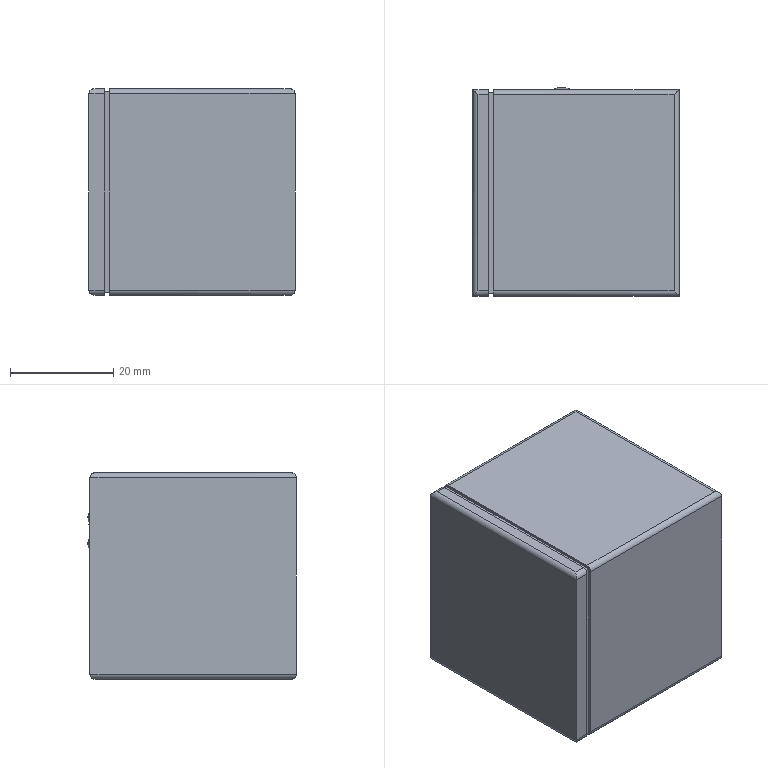Part | SolidWorks | features BaseBody 1 | 1 solid | 32 faces | box 40 x 40.45 x 40 mm | volume 63851 mm3 | plane 16 | cylinder 12 | spline 4 | commonest cylinder face diameters 2 x12
STEP:
#1=CARTESIAN_POINT('',(19.153,20.,6.3));
#2=VERTEX_POINT('',#1);
#3=CARTESIAN_POINT('',(15.347,20.,6.3));
#4=VERTEX_POINT('',#3);
#5=CARTESIAN_POINT('',(19.153,20.,6.3));
#6=CARTESIAN_POINT('',(19.153,20.,6.426));
#7=CARTESIAN_POINT('',(19.141,20.,6.549));
#8=CARTESIAN_POINT('',(19.093,20.,6.792));
#9=CARTESIAN_POINT('',(19.056,20.,6.913));
#10=CARTESIAN_POINT('',(18.961,20.,7.144));
#11=CARTESIAN_POINT('',(18.902,20.,7.253));
#12=CARTESIAN_POINT('',(18.764,20.,7.46));
#13=CARTESIAN_POINT('',(18.684,20.,7.558));
#14=CARTESIAN_POINT('',(18.421,20.,7.821));
#15=CARTESIAN_POINT('',(18.209,20.,7.963));
#16=CARTESIAN_POINT('',(17.751,20.,8.153));
#17=CARTESIAN_POINT('',(17.501,20.,8.203));
#18=CARTESIAN_POINT('',(17.124,20.,8.203));
#19=CARTESIAN_POINT('',(17.001,20.,8.191));
#20=CARTESIAN_POINT('',(16.758,20.,8.143));
#21=CARTESIAN_POINT('',(16.637,20.,8.106));
#22=CARTESIAN_POINT('',(16.406,20.,8.011));
#23=CARTESIAN_POINT('',(16.297,20.,7.952));
#24=CARTESIAN_POINT('',(16.09,20.,7.814));
#25=CARTESIAN_POINT('',(15.992,20.,7.734));
#26=CARTESIAN_POINT('',(15.729,20.,7.471));
#27=CARTESIAN_POINT('',(15.587,20.,7.259));
#28=CARTESIAN_POINT('',(15.397,20.,6.801));
#29=CARTESIAN_POINT('',(15.347,20.,6.551));
#30=CARTESIAN_POINT('',(15.347,20.,6.3));
#31=B_SPLINE_CURVE_WITH_KNOTS('',3,(#5,#6,#7,#8,#9,#10,#11,#12,#13,#14,#15,#16,#17,#18,#19,#20,#21,#22,#23,#24,#25,#26,#27,#28,#29,#30),.UNSPECIFIED.,.F.,.F.,(4,2,2,2,2,2,2,2,2,2,2,2,4),(0.,0.0003717,0.0007433,0.001115,0.001487,0.00223,0.002973,0.003345,0.003717,0.004088,0.00446,0.005203,0.005946),.UNSPECIFIED.);
#32=EDGE_CURVE('',#2,#4,#31,.T.);
#33=ORIENTED_EDGE('',*,*,#32,.F.);
#34=CARTESIAN_POINT('',(17.25,16.2,6.3));
#35=DIRECTION('',(0.,0.,1.));
#36=DIRECTION('',(1.,0.,0.));
#37=AXIS2_PLACEMENT_3D('',#34,#35,#36);
#38=CIRCLE('',#37,4.25);
#39=EDGE_CURVE('',#2,#4,#38,.T.);
#40=ORIENTED_EDGE('',*,*,#39,.T.);
#41=EDGE_LOOP('',(#33,#40));
#42=FACE_OUTER_BOUND('',#41,.T.);
#43=CARTESIAN_POINT('',(19.174,19.989,6.3));
#44=CARTESIAN_POINT('',(19.174,19.989,6.895));
#45=CARTESIAN_POINT('',(19.174,19.852,7.475));
#46=CARTESIAN_POINT('',(19.174,19.583,8.006));
#47=CARTESIAN_POINT('',(17.941,20.616,6.3));
#48=CARTESIAN_POINT('',(17.941,20.616,6.994));
#49=CARTESIAN_POINT('',(17.941,20.455,7.669));
#50=CARTESIAN_POINT('',(17.941,20.142,8.288));
#51=CARTESIAN_POINT('',(16.559,20.616,6.3));
#52=CARTESIAN_POINT('',(16.559,20.616,6.994));
#53=CARTESIAN_POINT('',(16.559,20.455,7.669));
#54=CARTESIAN_POINT('',(16.559,20.142,8.288));
#55=CARTESIAN_POINT('',(15.326,19.989,6.3));
#56=CARTESIAN_POINT('',(15.326,19.989,6.895));
#57=CARTESIAN_POINT('',(15.326,19.852,7.475));
#58=CARTESIAN_POINT('',(15.326,19.583,8.006));
#59=(BOUNDED_SURFACE()B_SPLINE_SURFACE(3,3,((#43,#44,#45,#46),(#47,#48,#49,#50),(#51,#52,#53,#54),(#55,#56,#57,#58)),.UNSPECIFIED.,.F.,.F.,.F.)B_SPLINE_SURFACE_WITH_KNOTS((4,4),(4,4),(0.,1.),(0.,1.),.UNSPECIFIED.)GEOMETRIC_REPRESENTATION_ITEM()RATIONAL_B_SPLINE_SURFACE(((1.,0.9819,0.9819,1.),(0.9277,0.9109,0.9109,0.9277),(0.9277,0.9109,0.9109,0.9277),(1.,0.9819,0.9819,1.)))REPRESENTATION_ITEM('')SURFACE());
#60=ADVANCED_FACE('',(#42),#59,.T.);
#61=CARTESIAN_POINT('',(19.153,20.,11.3));
#62=VERTEX_POINT('',#61);
#63=CARTESIAN_POINT('',(15.347,20.,11.3));
#64=VERTEX_POINT('',#63);
#65=CARTESIAN_POINT('',(19.153,20.,11.3));
#66=CARTESIAN_POINT('',(19.153,20.,11.426));
#67=CARTESIAN_POINT('',(19.141,20.,11.549));
#68=CARTESIAN_POINT('',(19.093,20.,11.792));
#69=CARTESIAN_POINT('',(19.056,20.,11.913));
#70=CARTESIAN_POINT('',(18.961,20.,12.144));
#71=CARTESIAN_POINT('',(18.902,20.,12.253));
#72=CARTESIAN_POINT('',(18.764,20.,12.46));
#73=CARTESIAN_POINT('',(18.684,20.,12.558));
#74=CARTESIAN_POINT('',(18.421,20.,12.821));
#75=CARTESIAN_POINT('',(18.209,20.,12.963));
#76=CARTESIAN_POINT('',(17.751,20.,13.153));
#77=CARTESIAN_POINT('',(17.501,20.,13.203));
#78=CARTESIAN_POINT('',(17.124,20.,13.203));
#79=CARTESIAN_POINT('',(17.001,20.,13.191));
#80=CARTESIAN_POINT('',(16.758,20.,13.143));
#81=CARTESIAN_POINT('',(16.637,20.,13.106));
#82=CARTESIAN_POINT('',(16.406,20.,13.011));
#83=CARTESIAN_POINT('',(16.297,20.,12.952));
#84=CARTESIAN_POINT('',(16.09,20.,12.814));
#85=CARTESIAN_POINT('',(15.992,20.,12.734));
#86=CARTESIAN_POINT('',(15.729,20.,12.471));
#87=CARTESIAN_POINT('',(15.587,20.,12.259));
#88=CARTESIAN_POINT('',(15.397,20.,11.801));
#89=CARTESIAN_POINT('',(15.347,20.,11.551));
#90=CARTESIAN_POINT('',(15.347,20.,11.3));
#91=B_SPLINE_CURVE_WITH_KNOTS('',3,(#65,#66,#67,#68,#69,#70,#71,#72,#73,#74,#75,#76,#77,#78,#79,#80,#81,#82,#83,#84,#85,#86,#87,#88,#89,#90),.UNSPECIFIED.,.F.,.F.,(4,2,2,2,2,2,2,2,2,2,2,2,4),(0.,0.0003717,0.0007433,0.001115,0.001487,0.00223,0.002973,0.003345,0.003717,0.004088,0.00446,0.005203,0.005946),.UNSPECIFIED.);
#92=EDGE_CURVE('',#62,#64,#91,.T.);
#93=ORIENTED_EDGE('',*,*,#92,.F.);
#94=CARTESIAN_POINT('',(17.25,16.2,11.3));
#95=DIRECTION('',(0.,0.,1.));
#96=DIRECTION('',(1.,0.,0.));
#97=AXIS2_PLACEMENT_3D('',#94,#95,#96);
#98=CIRCLE('',#97,4.25);
#99=EDGE_CURVE('',#62,#64,#98,.T.);
#100=ORIENTED_EDGE('',*,*,#99,.T.);
#101=EDGE_LOOP('',(#93,#100));
#102=FACE_OUTER_BOUND('',#101,.T.);
#103=CARTESIAN_POINT('',(19.174,19.989,11.3));
#104=CARTESIAN_POINT('',(19.174,19.989,11.895));
#105=CARTESIAN_POINT('',(19.174,19.852,12.475));
#106=CARTESIAN_POINT('',(19.174,19.583,13.006));
#107=CARTESIAN_POINT('',(17.941,20.616,11.3));
#108=CARTESIAN_POINT('',(17.941,20.616,11.994));
#109=CARTESIAN_POINT('',(17.941,20.455,12.669));
#110=CARTESIAN_POINT('',(17.941,20.142,13.288));
#111=CARTESIAN_POINT('',(16.559,20.616,11.3));
#112=CARTESIAN_POINT('',(16.559,20.616,11.994));
#113=CARTESIAN_POINT('',(16.559,20.455,12.669));
#114=CARTESIAN_POINT('',(16.559,20.142,13.288));
#115=CARTESIAN_POINT('',(15.326,19.989,11.3));
#116=CARTESIAN_POINT('',(15.326,19.989,11.895));
#117=CARTESIAN_POINT('',(15.326,19.852,12.475));
#118=CARTESIAN_POINT('',(15.326,19.583,13.006));
#119=(BOUNDED_SURFACE()B_SPLINE_SURFACE(3,3,((#103,#104,#105,#106),(#107,#108,#109,#110),(#111,#112,#113,#114),(#115,#116,#117,#118)),.UNSPECIFIED.,.F.,.F.,.F.)B_SPLINE_SURFACE_WITH_KNOTS((4,4),(4,4),(0.,1.),(0.,1.),.UNSPECIFIED.)GEOMETRIC_REPRESENTATION_ITEM()RATIONAL_B_SPLINE_SURFACE(((1.,0.9819,0.9819,1.),(0.9277,0.9109,0.9109,0.9277),(0.9277,0.9109,0.9109,0.9277),(1.,0.9819,0.9819,1.)))REPRESENTATION_ITEM('')SURFACE());
#120=ADVANCED_FACE('',(#102),#119,.T.);
#121=CARTESIAN_POINT('',(40.,20.,19.));
#122=VERTEX_POINT('',#121);
#123=CARTESIAN_POINT('',(40.,-20.,19.));
#124=VERTEX_POINT('',#123);
#125=CARTESIAN_POINT('',(40.,20.,19.));
#126=DIRECTION('',(0.,-1.,0.));
#127=VECTOR('',#126,1000.);
#128=LINE('',#125,#127);
#129=EDGE_CURVE('',#122,#124,#128,.T.);
#130=ORIENTED_EDGE('',*,*,#129,.T.);
#131=CARTESIAN_POINT('',(40.,-20.,-19.));
#132=VERTEX_POINT('',#131);
#133=CARTESIAN_POINT('',(40.,-20.,19.));
#134=DIRECTION('',(0.,0.,-1.));
#135=VECTOR('',#134,1000.);
#136=LINE('',#133,#135);
#137=EDGE_CURVE('',#124,#132,#136,.T.);
#138=ORIENTED_EDGE('',*,*,#137,.T.);
#139=CARTESIAN_POINT('',(40.,20.,-19.));
#140=VERTEX_POINT('',#139);
#141=CARTESIAN_POINT('',(40.,20.,-19.));
#142=DIRECTION('',(0.,1.,0.));
#143=VECTOR('',#142,1000.);
#144=LINE('',#141,#143);
#145=EDGE_CURVE('',#132,#140,#144,.T.);
#146=ORIENTED_EDGE('',*,*,#145,.T.);
#147=CARTESIAN_POINT('',(40.,20.,19.));
#148=DIRECTION('',(0.,0.,1.));
#149=VECTOR('',#148,1000.);
#150=LINE('',#147,#149);
#151=EDGE_CURVE('',#140,#122,#150,.T.);
#152=ORIENTED_EDGE('',*,*,#151,.T.);
#153=EDGE_LOOP('',(#130,#138,#146,#152));
#154=FACE_OUTER_BOUND('',#153,.T.);
#155=CARTESIAN_POINT('',(40.,20.,19.));
#156=DIRECTION('',(1.,0.,0.));
#157=DIRECTION('',(0.,0.,-1.));
#158=AXIS2_PLACEMENT_3D('',#155,#156,#157);
#159=PLANE('',#158);
#160=ADVANCED_FACE('',(#154),#159,.T.);
#161=ORIENTED_EDGE('',*,*,#137,.F.);
#162=CARTESIAN_POINT('',(4.,-20.,19.));
#163=VERTEX_POINT('',#162);
#164=CARTESIAN_POINT('',(0.,-20.,19.));
#165=DIRECTION('',(1.,0.,0.));
#166=VECTOR('',#165,1000.);
#167=LINE('',#164,#166);
#168=EDGE_CURVE('',#163,#124,#167,.T.);
#169=ORIENTED_EDGE('',*,*,#168,.F.);
#170=CARTESIAN_POINT('',(4.,-20.,-19.));
#171=VERTEX_POINT('',#170);
#172=CARTESIAN_POINT('',(4.,-20.,0.));
#173=DIRECTION('',(0.,0.,1.));
#174=VECTOR('',#173,1000.);
#175=LINE('',#172,#174);
#176=EDGE_CURVE('',#171,#163,#175,.T.);
#177=ORIENTED_EDGE('',*,*,#176,.F.);
#178=CARTESIAN_POINT('',(0.,-20.,-19.));
#179=DIRECTION('',(-1.,0.,0.));
#180=VECTOR('',#179,1000.);
#181=LINE('',#178,#180);
#182=EDGE_CURVE('',#132,#171,#181,.T.);
#183=ORIENTED_EDGE('',*,*,#182,.F.);
#184=EDGE_LOOP('',(#161,#169,#177,#183));
#185=FACE_OUTER_BOUND('',#184,.T.);
#186=CARTESIAN_POINT('',(0.,-20.,0.));
#187=DIRECTION('',(0.,1.,0.));
#188=DIRECTION('',(0.,0.,1.));
#189=AXIS2_PLACEMENT_3D('',#186,#187,#188);
#190=PLANE('',#189);
#191=ADVANCED_FACE('',(#185),#190,.F.);
#192=ORIENTED_EDGE('',*,*,#129,.F.);
#193=CARTESIAN_POINT('',(39.,19.,20.));
#194=VERTEX_POINT('',#193);
#195=CARTESIAN_POINT('',(40.,20.,19.));
#196=CARTESIAN_POINT('',(40.,20.,19.586));
#197=CARTESIAN_POINT('',(39.586,19.586,20.));
#198=CARTESIAN_POINT('',(39.,19.,20.));
#199=(BOUNDED_CURVE()B_SPLINE_CURVE(3,(#195,#196,#197,#198),.UNSPECIFIED.,.F.,.F.)B_SPLINE_CURVE_WITH_KNOTS((4,4),(0.,1.571),.UNSPECIFIED.)CURVE()GEOMETRIC_REPRESENTATION_ITEM()RATIONAL_B_SPLINE_CURVE((1.,0.8047,0.8047,1.))REPRESENTATION_ITEM(''));
#200=EDGE_CURVE('',#122,#194,#199,.T.);
#201=ORIENTED_EDGE('',*,*,#200,.T.);
#202=CARTESIAN_POINT('',(39.,-19.,20.));
#203=VERTEX_POINT('',#202);
#204=CARTESIAN_POINT('',(39.,20.,20.));
#205=DIRECTION('',(0.,-1.,0.));
#206=VECTOR('',#205,1000.);
#207=LINE('',#204,#206);
#208=EDGE_CURVE('',#194,#203,#207,.T.);
#209=ORIENTED_EDGE('',*,*,#208,.T.);
#210=CARTESIAN_POINT('',(39.,-19.,20.));
#211=CARTESIAN_POINT('',(39.586,-19.586,20.));
#212=CARTESIAN_POINT('',(40.,-20.,19.586));
#213=CARTESIAN_POINT('',(40.,-20.,19.));
#214=(BOUNDED_CURVE()B_SPLINE_CURVE(3,(#210,#211,#212,#213),.UNSPECIFIED.,.F.,.F.)B_SPLINE_CURVE_WITH_KNOTS((4,4),(1.571,3.142),.UNSPECIFIED.)CURVE()GEOMETRIC_REPRESENTATION_ITEM()RATIONAL_B_SPLINE_CURVE((1.,0.8047,0.8047,1.))REPRESENTATION_ITEM(''));
#215=EDGE_CURVE('',#203,#124,#214,.T.);
#216=ORIENTED_EDGE('',*,*,#215,.T.);
#217=EDGE_LOOP('',(#192,#201,#209,#216));
#218=FACE_OUTER_BOUND('',#217,.T.);
#219=CARTESIAN_POINT('',(39.,20.,19.));
#220=DIRECTION('',(0.,1.,0.));
#221=DIRECTION('',(0.,0.,1.));
#222=AXIS2_PLACEMENT_3D('',#219,#220,#221);
#223=CYLINDRICAL_SURFACE('',#222,1.);
#224=ADVANCED_FACE('',(#218),#223,.T.);
#225=CARTESIAN_POINT('',(15.347,20.,6.3));
#226=CARTESIAN_POINT('',(15.347,20.,6.174));
#227=CARTESIAN_POINT('',(15.359,20.,6.051));
#228=CARTESIAN_POINT('',(15.407,20.,5.807));
#229=CARTESIAN_POINT('',(15.444,20.,5.687));
#230=CARTESIAN_POINT('',(15.539,20.,5.456));
#231=CARTESIAN_POINT('',(15.598,20.,5.347));
#232=CARTESIAN_POINT('',(15.736,20.,5.14));
#233=CARTESIAN_POINT('',(15.816,20.,5.042));
#234=CARTESIAN_POINT('',(16.08,20.,4.779));
#235=CARTESIAN_POINT('',(16.292,20.,4.637));
#236=CARTESIAN_POINT('',(16.75,20.,4.447));
#237=CARTESIAN_POINT('',(17.,20.,4.397));
#238=CARTESIAN_POINT('',(17.373,20.,4.397));
#239=CARTESIAN_POINT('',(17.499,20.,4.409));
#240=CARTESIAN_POINT('',(17.743,20.,4.457));
#241=CARTESIAN_POINT('',(17.862,20.,4.493));
#242=CARTESIAN_POINT('',(18.092,20.,4.589));
#243=CARTESIAN_POINT('',(18.204,20.,4.648));
#244=CARTESIAN_POINT('',(18.41,20.,4.786));
#245=CARTESIAN_POINT('',(18.506,20.,4.864));
#246=CARTESIAN_POINT('',(18.684,20.,5.042));
#247=CARTESIAN_POINT('',(18.763,20.,5.138));
#248=CARTESIAN_POINT('',(18.901,20.,5.344));
#249=CARTESIAN_POINT('',(18.96,20.,5.455));
#250=CARTESIAN_POINT('',(19.056,20.,5.686));
#251=CARTESIAN_POINT('',(19.092,20.,5.805));
#252=CARTESIAN_POINT('',(19.141,20.,6.048));
#253=CARTESIAN_POINT('',(19.153,20.,6.174));
#254=CARTESIAN_POINT('',(19.153,20.,6.3));
#255=B_SPLINE_CURVE_WITH_KNOTS('',3,(#225,#226,#227,#228,#229,#230,#231,#232,#233,#234,#235,#236,#237,#238,#239,#240,#241,#242,#243,#244,#245,#246,#247,#248,#249,#250,#251,#252,#253,#254),.UNSPECIFIED.,.F.,.F.,(4,2,2,2,2,2,2,2,2,2,2,2,2,2,4),(-0.005949,-0.005577,-0.005206,-0.004834,-0.004462,-0.003718,-0.002975,-0.002603,-0.002231,-0.001859,-0.001487,-0.001115,-0.0007437,-0.0003718,0.),.UNSPECIFIED.);
#256=EDGE_CURVE('',#4,#2,#255,.T.);
#257=ORIENTED_EDGE('',*,*,#256,.T.);
#258=ORIENTED_EDGE('',*,*,#32,.T.);
#259=EDGE_LOOP('',(#257,#258));
#260=FACE_BOUND('',#259,.T.);
#261=CARTESIAN_POINT('',(15.347,20.,11.3));
#262=CARTESIAN_POINT('',(15.347,20.,11.174));
#263=CARTESIAN_POINT('',(15.359,20.,11.051));
#264=CARTESIAN_POINT('',(15.407,20.,10.807));
#265=CARTESIAN_POINT('',(15.444,20.,10.687));
#266=CARTESIAN_POINT('',(15.539,20.,10.456));
#267=CARTESIAN_POINT('',(15.598,20.,10.347));
#268=CARTESIAN_POINT('',(15.736,20.,10.14));
#269=CARTESIAN_POINT('',(15.816,20.,10.042));
#270=CARTESIAN_POINT('',(16.08,20.,9.779));
#271=CARTESIAN_POINT('',(16.292,20.,9.637));
#272=CARTESIAN_POINT('',(16.75,20.,9.447));
#273=CARTESIAN_POINT('',(17.,20.,9.397));
#274=CARTESIAN_POINT('',(17.373,20.,9.397));
#275=CARTESIAN_POINT('',(17.499,20.,9.409));
#276=CARTESIAN_POINT('',(17.743,20.,9.457));
#277=CARTESIAN_POINT('',(17.862,20.,9.493));
#278=CARTESIAN_POINT('',(18.092,20.,9.589));
#279=CARTESIAN_POINT('',(18.204,20.,9.648));
#280=CARTESIAN_POINT('',(18.41,20.,9.786));
#281=CARTESIAN_POINT('',(18.506,20.,9.864));
#282=CARTESIAN_POINT('',(18.684,20.,10.042));
#283=CARTESIAN_POINT('',(18.763,20.,10.138));
#284=CARTESIAN_POINT('',(18.901,20.,10.344));
#285=CARTESIAN_POINT('',(18.96,20.,10.455));
#286=CARTESIAN_POINT('',(19.056,20.,10.686));
#287=CARTESIAN_POINT('',(19.092,20.,10.805));
#288=CARTESIAN_POINT('',(19.141,20.,11.048));
#289=CARTESIAN_POINT('',(19.153,20.,11.174));
#290=CARTESIAN_POINT('',(19.153,20.,11.3));
#291=B_SPLINE_CURVE_WITH_KNOTS('',3,(#261,#262,#263,#264,#265,#266,#267,#268,#269,#270,#271,#272,#273,#274,#275,#276,#277,#278,#279,#280,#281,#282,#283,#284,#285,#286,#287,#288,#289,#290),.UNSPECIFIED.,.F.,.F.,(4,2,2,2,2,2,2,2,2,2,2,2,2,2,4),(-0.005949,-0.005577,-0.005206,-0.004834,-0.004462,-0.003718,-0.002975,-0.002603,-0.002231,-0.001859,-0.001487,-0.001115,-0.0007437,-0.0003718,0.),.UNSPECIFIED.);
#292=EDGE_CURVE('',#64,#62,#291,.T.);
#293=ORIENTED_EDGE('',*,*,#292,.T.);
#294=ORIENTED_EDGE('',*,*,#92,.T.);
#295=EDGE_LOOP('',(#293,#294));
#296=FACE_BOUND('',#295,.T.);
#297=CARTESIAN_POINT('',(4.,20.,-19.));
#298=VERTEX_POINT('',#297);
#299=CARTESIAN_POINT('',(0.,20.,-19.));
#300=DIRECTION('',(-1.,0.,0.));
#301=VECTOR('',#300,1000.);
#302=LINE('',#299,#301);
#303=EDGE_CURVE('',#140,#298,#302,.T.);
#304=ORIENTED_EDGE('',*,*,#303,.T.);
#305=CARTESIAN_POINT('',(4.,20.,19.));
#306=VERTEX_POINT('',#305);
#307=CARTESIAN_POINT('',(4.,20.,0.));
#308=DIRECTION('',(0.,0.,1.));
#309=VECTOR('',#308,1000.);
#310=LINE('',#307,#309);
#311=EDGE_CURVE('',#298,#306,#310,.T.);
#312=ORIENTED_EDGE('',*,*,#311,.T.);
#313=CARTESIAN_POINT('',(0.,20.,19.));
#314=DIRECTION('',(1.,0.,0.));
#315=VECTOR('',#314,1000.);
#316=LINE('',#313,#315);
#317=EDGE_CURVE('',#306,#122,#316,.T.);
#318=ORIENTED_EDGE('',*,*,#317,.T.);
#319=ORIENTED_EDGE('',*,*,#151,.F.);
#320=EDGE_LOOP('',(#304,#312,#318,#319));
#321=FACE_OUTER_BOUND('',#320,.T.);
#322=CARTESIAN_POINT('',(0.,20.,0.));
#323=DIRECTION('',(0.,1.,0.));
#324=DIRECTION('',(0.,0.,1.));
#325=AXIS2_PLACEMENT_3D('',#322,#323,#324);
#326=PLANE('',#325);
#327=ADVANCED_FACE('',(#260,#296,#321),#326,.T.);
#328=CARTESIAN_POINT('',(39.,-19.,-20.));
#329=VERTEX_POINT('',#328);
#330=CARTESIAN_POINT('',(39.,19.,-20.));
#331=VERTEX_POINT('',#330);
#332=CARTESIAN_POINT('',(39.,20.,-20.));
#333=DIRECTION('',(0.,1.,0.));
#334=VECTOR('',#333,1000.);
#335=LINE('',#332,#334);
#336=EDGE_CURVE('',#329,#331,#335,.T.);
#337=ORIENTED_EDGE('',*,*,#336,.T.);
#338=CARTESIAN_POINT('',(39.,19.,-20.));
#339=CARTESIAN_POINT('',(39.586,19.586,-20.));
#340=CARTESIAN_POINT('',(40.,20.,-19.586));
#341=CARTESIAN_POINT('',(40.,20.,-19.));
#342=(BOUNDED_CURVE()B_SPLINE_CURVE(3,(#338,#339,#340,#341),.UNSPECIFIED.,.F.,.F.)B_SPLINE_CURVE_WITH_KNOTS((4,4),(4.712,6.283),.UNSPECIFIED.)CURVE()GEOMETRIC_REPRESENTATION_ITEM()RATIONAL_B_SPLINE_CURVE((1.,0.8047,0.8047,1.))REPRESENTATION_ITEM(''));
#343=EDGE_CURVE('',#331,#140,#342,.T.);
#344=ORIENTED_EDGE('',*,*,#343,.T.);
#345=ORIENTED_EDGE('',*,*,#145,.F.);
#346=CARTESIAN_POINT('',(40.,-20.,-19.));
#347=CARTESIAN_POINT('',(40.,-20.,-19.586));
#348=CARTESIAN_POINT('',(39.586,-19.586,-20.));
#349=CARTESIAN_POINT('',(39.,-19.,-20.));
#350=(BOUNDED_CURVE()B_SPLINE_CURVE(3,(#346,#347,#348,#349),.UNSPECIFIED.,.F.,.F.)B_SPLINE_CURVE_WITH_KNOTS((4,4),(3.142,4.712),.UNSPECIFIED.)CURVE()GEOMETRIC_REPRESENTATION_ITEM()RATIONAL_B_SPLINE_CURVE((1.,0.8047,0.8047,1.))REPRESENTATION_ITEM(''));
#351=EDGE_CURVE('',#132,#329,#350,.T.);
#352=ORIENTED_EDGE('',*,*,#351,.T.);
#353=EDGE_LOOP('',(#337,#344,#345,#352));
#354=FACE_OUTER_BOUND('',#353,.T.);
#355=CARTESIAN_POINT('',(39.,20.,-19.));
#356=DIRECTION('',(0.,1.,0.));
#357=DIRECTION('',(0.,0.,1.));
#358=AXIS2_PLACEMENT_3D('',#355,#356,#357);
#359=CYLINDRICAL_SURFACE('',#358,1.);
#360=ADVANCED_FACE('',(#354),#359,.T.);
#361=ORIENTED_EDGE('',*,*,#182,.T.);
#362=CARTESIAN_POINT('',(4.,-19.,-20.));
#363=VERTEX_POINT('',#362);
#364=CARTESIAN_POINT('',(4.,-19.,-19.));
#365=DIRECTION('',(1.,0.,0.));
#366=DIRECTION('',(0.,0.,1.));
#367=AXIS2_PLACEMENT_3D('',#364,#365,#366);
#368=CIRCLE('',#367,1.);
#369=EDGE_CURVE('',#171,#363,#368,.T.);
#370=ORIENTED_EDGE('',*,*,#369,.T.);
#371=CARTESIAN_POINT('',(0.,-19.,-20.));
#372=DIRECTION('',(1.,0.,0.));
#373=VECTOR('',#372,1000.);
#374=LINE('',#371,#373);
#375=EDGE_CURVE('',#363,#329,#374,.T.);
#376=ORIENTED_EDGE('',*,*,#375,.T.);
#377=ORIENTED_EDGE('',*,*,#351,.F.);
#378=EDGE_LOOP('',(#361,#370,#376,#377));
#379=FACE_OUTER_BOUND('',#378,.T.);
#380=CARTESIAN_POINT('',(0.,-19.,-19.));
#381=DIRECTION('',(-1.,0.,0.));
#382=DIRECTION('',(0.,0.,1.));
#383=AXIS2_PLACEMENT_3D('',#380,#381,#382);
#384=CYLINDRICAL_SURFACE('',#383,1.);
#385=ADVANCED_FACE('',(#379),#384,.T.);
#386=CARTESIAN_POINT('',(4.,-19.,20.));
#387=VERTEX_POINT('',#386);
#388=CARTESIAN_POINT('',(0.,-19.,20.));
#389=DIRECTION('',(-1.,0.,0.));
#390=VECTOR('',#389,1000.);
#391=LINE('',#388,#390);
#392=EDGE_CURVE('',#203,#387,#391,.T.);
#393=ORIENTED_EDGE('',*,*,#392,.T.);
#394=CARTESIAN_POINT('',(4.,-19.,19.));
#395=DIRECTION('',(1.,0.,0.));
#396=DIRECTION('',(0.,0.,1.));
#397=AXIS2_PLACEMENT_3D('',#394,#395,#396);
#398=CIRCLE('',#397,1.);
#399=EDGE_CURVE('',#387,#163,#398,.T.);
#400=ORIENTED_EDGE('',*,*,#399,.T.);
#401=ORIENTED_EDGE('',*,*,#168,.T.);
#402=ORIENTED_EDGE('',*,*,#215,.F.);
#403=EDGE_LOOP('',(#393,#400,#401,#402));
#404=FACE_OUTER_BOUND('',#403,.T.);
#405=CARTESIAN_POINT('',(0.,-19.,19.));
#406=DIRECTION('',(-1.,0.,0.));
#407=DIRECTION('',(0.,0.,1.));
#408=AXIS2_PLACEMENT_3D('',#405,#406,#407);
#409=CYLINDRICAL_SURFACE('',#408,1.);
#410=ADVANCED_FACE('',(#404),#409,.T.);
#411=CARTESIAN_POINT('',(4.,19.45,19.45));
#412=VERTEX_POINT('',#411);
#413=CARTESIAN_POINT('',(4.,19.45,-19.45));
#414=VERTEX_POINT('',#413);
#415=CARTESIAN_POINT('',(4.,19.45,0.));
#416=DIRECTION('',(0.,0.,-1.));
#417=VECTOR('',#416,1000.);
#418=LINE('',#415,#417);
#419=EDGE_CURVE('',#412,#414,#418,.T.);
#420=ORIENTED_EDGE('',*,*,#419,.F.);
#421=CARTESIAN_POINT('',(4.,-19.45,19.45));
#422=VERTEX_POINT('',#421);
#423=CARTESIAN_POINT('',(4.,0.,19.45));
#424=DIRECTION('',(0.,1.,0.));
#425=VECTOR('',#424,1000.);
#426=LINE('',#423,#425);
#427=EDGE_CURVE('',#422,#412,#426,.T.);
#428=ORIENTED_EDGE('',*,*,#427,.F.);
#429=CARTESIAN_POINT('',(4.,-19.45,-19.45));
#430=VERTEX_POINT('',#429);
#431=CARTESIAN_POINT('',(4.,-19.45,0.));
#432=DIRECTION('',(0.,0.,1.));
#433=VECTOR('',#432,1000.);
#434=LINE('',#431,#433);
#435=EDGE_CURVE('',#430,#422,#434,.T.);
#436=ORIENTED_EDGE('',*,*,#435,.F.);
#437=CARTESIAN_POINT('',(4.,0.,-19.45));
#438=DIRECTION('',(0.,-1.,0.));
#439=VECTOR('',#438,1000.);
#440=LINE('',#437,#439);
#441=EDGE_CURVE('',#414,#430,#440,.T.);
#442=ORIENTED_EDGE('',*,*,#441,.F.);
#443=EDGE_LOOP('',(#420,#428,#436,#442));
#444=FACE_BOUND('',#443,.T.);
#445=CARTESIAN_POINT('',(4.,19.,-20.));
#446=VERTEX_POINT('',#445);
#447=CARTESIAN_POINT('',(4.,19.,-19.));
#448=DIRECTION('',(1.,0.,0.));
#449=DIRECTION('',(0.,0.,1.));
#450=AXIS2_PLACEMENT_3D('',#447,#448,#449);
#451=CIRCLE('',#450,1.);
#452=EDGE_CURVE('',#446,#298,#451,.T.);
#453=ORIENTED_EDGE('',*,*,#452,.F.);
#454=CARTESIAN_POINT('',(4.,0.,-20.));
#455=DIRECTION('',(0.,1.,0.));
#456=VECTOR('',#455,1000.);
#457=LINE('',#454,#456);
#458=EDGE_CURVE('',#363,#446,#457,.T.);
#459=ORIENTED_EDGE('',*,*,#458,.F.);
#460=ORIENTED_EDGE('',*,*,#369,.F.);
#461=ORIENTED_EDGE('',*,*,#176,.T.);
#462=ORIENTED_EDGE('',*,*,#399,.F.);
#463=CARTESIAN_POINT('',(4.,19.,20.));
#464=VERTEX_POINT('',#463);
#465=CARTESIAN_POINT('',(4.,0.,20.));
#466=DIRECTION('',(0.,-1.,0.));
#467=VECTOR('',#466,1000.);
#468=LINE('',#465,#467);
#469=EDGE_CURVE('',#464,#387,#468,.T.);
#470=ORIENTED_EDGE('',*,*,#469,.F.);
#471=CARTESIAN_POINT('',(4.,19.,19.));
#472=DIRECTION('',(1.,0.,0.));
#473=DIRECTION('',(0.,0.,1.));
#474=AXIS2_PLACEMENT_3D('',#471,#472,#473);
#475=CIRCLE('',#474,1.);
#476=EDGE_CURVE('',#306,#464,#475,.T.);
#477=ORIENTED_EDGE('',*,*,#476,.F.);
#478=ORIENTED_EDGE('',*,*,#311,.F.);
#479=EDGE_LOOP('',(#453,#459,#460,#461,#462,#470,#477,#478));
#480=FACE_OUTER_BOUND('',#479,.T.);
#481=CARTESIAN_POINT('',(4.,0.,0.));
#482=DIRECTION('',(1.,0.,0.));
#483=DIRECTION('',(0.,0.,-1.));
#484=AXIS2_PLACEMENT_3D('',#481,#482,#483);
#485=PLANE('',#484);
#486=ADVANCED_FACE('',(#444,#480),#485,.F.);
#487=ORIENTED_EDGE('',*,*,#317,.F.);
#488=ORIENTED_EDGE('',*,*,#476,.T.);
#489=CARTESIAN_POINT('',(0.,19.,20.));
#490=DIRECTION('',(1.,0.,0.));
#491=VECTOR('',#490,1000.);
#492=LINE('',#489,#491);
#493=EDGE_CURVE('',#464,#194,#492,.T.);
#494=ORIENTED_EDGE('',*,*,#493,.T.);
#495=ORIENTED_EDGE('',*,*,#200,.F.);
#496=EDGE_LOOP('',(#487,#488,#494,#495));
#497=FACE_OUTER_BOUND('',#496,.T.);
#498=CARTESIAN_POINT('',(0.,19.,19.));
#499=DIRECTION('',(-1.,0.,0.));
#500=DIRECTION('',(0.,0.,1.));
#501=AXIS2_PLACEMENT_3D('',#498,#499,#500);
#502=CYLINDRICAL_SURFACE('',#501,1.);
#503=ADVANCED_FACE('',(#497),#502,.T.);
#504=ORIENTED_EDGE('',*,*,#493,.F.);
#505=ORIENTED_EDGE('',*,*,#469,.T.);
#506=ORIENTED_EDGE('',*,*,#392,.F.);
#507=ORIENTED_EDGE('',*,*,#208,.F.);
#508=EDGE_LOOP('',(#504,#505,#506,#507));
#509=FACE_OUTER_BOUND('',#508,.T.);
#510=CARTESIAN_POINT('',(1.,20.,20.));
#511=DIRECTION('',(0.,0.,1.));
#512=DIRECTION('',(1.,0.,0.));
#513=AXIS2_PLACEMENT_3D('',#510,#511,#512);
#514=PLANE('',#513);
#515=ADVANCED_FACE('',(#509),#514,.T.);
#516=ORIENTED_EDGE('',*,*,#39,.F.);
#517=ORIENTED_EDGE('',*,*,#256,.F.);
#518=EDGE_LOOP('',(#516,#517));
#519=FACE_OUTER_BOUND('',#518,.T.);
#520=CARTESIAN_POINT('',(19.174,19.579,4.585));
#521=CARTESIAN_POINT('',(19.174,19.85,5.119));
#522=CARTESIAN_POINT('',(19.174,19.989,5.701));
#523=CARTESIAN_POINT('',(19.174,19.989,6.3));
#524=CARTESIAN_POINT('',(17.941,20.137,4.302));
#525=CARTESIAN_POINT('',(17.941,20.453,4.924));
#526=CARTESIAN_POINT('',(17.941,20.616,5.602));
#527=CARTESIAN_POINT('',(17.941,20.616,6.3));
#528=CARTESIAN_POINT('',(16.559,20.137,4.302));
#529=CARTESIAN_POINT('',(16.559,20.453,4.924));
#530=CARTESIAN_POINT('',(16.559,20.616,5.602));
#531=CARTESIAN_POINT('',(16.559,20.616,6.3));
#532=CARTESIAN_POINT('',(15.326,19.579,4.585));
#533=CARTESIAN_POINT('',(15.326,19.85,5.119));
#534=CARTESIAN_POINT('',(15.326,19.989,5.701));
#535=CARTESIAN_POINT('',(15.326,19.989,6.3));
#536=(BOUNDED_SURFACE()B_SPLINE_SURFACE(3,3,((#520,#521,#522,#523),(#524,#525,#526,#527),(#528,#529,#530,#531),(#532,#533,#534,#535)),.UNSPECIFIED.,.F.,.F.,.F.)B_SPLINE_SURFACE_WITH_KNOTS((4,4),(4,4),(0.,1.),(0.,1.),.UNSPECIFIED.)GEOMETRIC_REPRESENTATION_ITEM()RATIONAL_B_SPLINE_SURFACE(((1.,0.9817,0.9817,1.),(0.9277,0.9108,0.9108,0.9277),(0.9277,0.9108,0.9108,0.9277),(1.,0.9817,0.9817,1.)))REPRESENTATION_ITEM('')SURFACE());
#537=ADVANCED_FACE('',(#519),#536,.T.);
#538=ORIENTED_EDGE('',*,*,#99,.F.);
#539=ORIENTED_EDGE('',*,*,#292,.F.);
#540=EDGE_LOOP('',(#538,#539));
#541=FACE_OUTER_BOUND('',#540,.T.);
#542=CARTESIAN_POINT('',(19.174,19.579,9.585));
#543=CARTESIAN_POINT('',(19.174,19.85,10.119));
#544=CARTESIAN_POINT('',(19.174,19.989,10.701));
#545=CARTESIAN_POINT('',(19.174,19.989,11.3));
#546=CARTESIAN_POINT('',(17.941,20.137,9.302));
#547=CARTESIAN_POINT('',(17.941,20.453,9.924));
#548=CARTESIAN_POINT('',(17.941,20.616,10.602));
#549=CARTESIAN_POINT('',(17.941,20.616,11.3));
#550=CARTESIAN_POINT('',(16.559,20.137,9.302));
#551=CARTESIAN_POINT('',(16.559,20.453,9.924));
#552=CARTESIAN_POINT('',(16.559,20.616,10.602));
#553=CARTESIAN_POINT('',(16.559,20.616,11.3));
#554=CARTESIAN_POINT('',(15.326,19.579,9.585));
#555=CARTESIAN_POINT('',(15.326,19.85,10.119));
#556=CARTESIAN_POINT('',(15.326,19.989,10.701));
#557=CARTESIAN_POINT('',(15.326,19.989,11.3));
#558=(BOUNDED_SURFACE()B_SPLINE_SURFACE(3,3,((#542,#543,#544,#545),(#546,#547,#548,#549),(#550,#551,#552,#553),(#554,#555,#556,#557)),.UNSPECIFIED.,.F.,.F.,.F.)B_SPLINE_SURFACE_WITH_KNOTS((4,4),(4,4),(0.,1.),(0.,1.),.UNSPECIFIED.)GEOMETRIC_REPRESENTATION_ITEM()RATIONAL_B_SPLINE_SURFACE(((1.,0.9817,0.9817,1.),(0.9277,0.9108,0.9108,0.9277),(0.9277,0.9108,0.9108,0.9277),(1.,0.9817,0.9817,1.)))REPRESENTATION_ITEM('')SURFACE());
#559=ADVANCED_FACE('',(#541),#558,.T.);
#560=CARTESIAN_POINT('',(0.,19.,-20.));
#561=DIRECTION('',(-1.,0.,0.));
#562=VECTOR('',#561,1000.);
#563=LINE('',#560,#562);
#564=EDGE_CURVE('',#331,#446,#563,.T.);
#565=ORIENTED_EDGE('',*,*,#564,.T.);
#566=ORIENTED_EDGE('',*,*,#452,.T.);
#567=ORIENTED_EDGE('',*,*,#303,.F.);
#568=ORIENTED_EDGE('',*,*,#343,.F.);
#569=EDGE_LOOP('',(#565,#566,#567,#568));
#570=FACE_OUTER_BOUND('',#569,.T.);
#571=CARTESIAN_POINT('',(0.,19.,-19.));
#572=DIRECTION('',(-1.,0.,0.));
#573=DIRECTION('',(0.,0.,1.));
#574=AXIS2_PLACEMENT_3D('',#571,#572,#573);
#575=CYLINDRICAL_SURFACE('',#574,1.);
#576=ADVANCED_FACE('',(#570),#575,.T.);
#577=ORIENTED_EDGE('',*,*,#375,.F.);
#578=ORIENTED_EDGE('',*,*,#458,.T.);
#579=ORIENTED_EDGE('',*,*,#564,.F.);
#580=ORIENTED_EDGE('',*,*,#336,.F.);
#581=EDGE_LOOP('',(#577,#578,#579,#580));
#582=FACE_OUTER_BOUND('',#581,.T.);
#583=CARTESIAN_POINT('',(39.,20.,-20.));
#584=DIRECTION('',(0.,0.,-1.));
#585=DIRECTION('',(-1.,0.,0.));
#586=AXIS2_PLACEMENT_3D('',#583,#584,#585);
#587=PLANE('',#586);
#588=ADVANCED_FACE('',(#582),#587,.T.);
#589=CARTESIAN_POINT('',(3.,19.45,-19.45));
#590=VERTEX_POINT('',#589);
#591=CARTESIAN_POINT('',(3.,-19.45,-19.45));
#592=VERTEX_POINT('',#591);
#593=CARTESIAN_POINT('',(3.,-19.45,-19.45));
#594=DIRECTION('',(0.,-1.,0.));
#595=VECTOR('',#594,1000.);
#596=LINE('',#593,#595);
#597=EDGE_CURVE('',#590,#592,#596,.T.);
#598=ORIENTED_EDGE('',*,*,#597,.F.);
#599=CARTESIAN_POINT('',(3.,19.45,-19.45));
#600=DIRECTION('',(-1.,0.,0.));
#601=VECTOR('',#600,1000.);
#602=LINE('',#599,#601);
#603=EDGE_CURVE('',#414,#590,#602,.T.);
#604=ORIENTED_EDGE('',*,*,#603,.F.);
#605=ORIENTED_EDGE('',*,*,#441,.T.);
#606=CARTESIAN_POINT('',(3.,-19.45,-19.45));
#607=DIRECTION('',(1.,0.,0.));
#608=VECTOR('',#607,1000.);
#609=LINE('',#606,#608);
#610=EDGE_CURVE('',#592,#430,#609,.T.);
#611=ORIENTED_EDGE('',*,*,#610,.F.);
#612=EDGE_LOOP('',(#598,#604,#605,#611));
#613=FACE_OUTER_BOUND('',#612,.T.);
#614=CARTESIAN_POINT('',(3.,-19.45,-19.45));
#615=DIRECTION('',(0.,0.,1.));
#616=DIRECTION('',(1.,0.,0.));
#617=AXIS2_PLACEMENT_3D('',#614,#615,#616);
#618=PLANE('',#617);
#619=ADVANCED_FACE('',(#613),#618,.F.);
#620=CARTESIAN_POINT('',(3.,19.45,19.45));
#621=VERTEX_POINT('',#620);
#622=CARTESIAN_POINT('',(3.,19.45,-19.45));
#623=DIRECTION('',(0.,0.,-1.));
#624=VECTOR('',#623,1000.);
#625=LINE('',#622,#624);
#626=EDGE_CURVE('',#621,#590,#625,.T.);
#627=ORIENTED_EDGE('',*,*,#626,.F.);
#628=CARTESIAN_POINT('',(3.,19.45,19.45));
#629=DIRECTION('',(-1.,0.,0.));
#630=VECTOR('',#629,1000.);
#631=LINE('',#628,#630);
#632=EDGE_CURVE('',#412,#621,#631,.T.);
#633=ORIENTED_EDGE('',*,*,#632,.F.);
#634=ORIENTED_EDGE('',*,*,#419,.T.);
#635=ORIENTED_EDGE('',*,*,#603,.T.);
#636=EDGE_LOOP('',(#627,#633,#634,#635));
#637=FACE_OUTER_BOUND('',#636,.T.);
#638=CARTESIAN_POINT('',(3.,19.45,-19.45));
#639=DIRECTION('',(0.,-1.,0.));
#640=DIRECTION('',(0.,0.,-1.));
#641=AXIS2_PLACEMENT_3D('',#638,#639,#640);
#642=PLANE('',#641);
#643=ADVANCED_FACE('',(#637),#642,.F.);
#644=CARTESIAN_POINT('',(3.,-19.45,19.45));
#645=VERTEX_POINT('',#644);
#646=CARTESIAN_POINT('',(3.,19.45,19.45));
#647=DIRECTION('',(0.,1.,0.));
#648=VECTOR('',#647,1000.);
#649=LINE('',#646,#648);
#650=EDGE_CURVE('',#645,#621,#649,.T.);
#651=ORIENTED_EDGE('',*,*,#650,.F.);
#652=CARTESIAN_POINT('',(3.,-19.45,19.45));
#653=DIRECTION('',(-1.,0.,0.));
#654=VECTOR('',#653,1000.);
#655=LINE('',#652,#654);
#656=EDGE_CURVE('',#422,#645,#655,.T.);
#657=ORIENTED_EDGE('',*,*,#656,.F.);
#658=ORIENTED_EDGE('',*,*,#427,.T.);
#659=ORIENTED_EDGE('',*,*,#632,.T.);
#660=EDGE_LOOP('',(#651,#657,#658,#659));
#661=FACE_OUTER_BOUND('',#660,.T.);
#662=CARTESIAN_POINT('',(3.,19.45,19.45));
#663=DIRECTION('',(0.,0.,-1.));
#664=DIRECTION('',(-1.,0.,0.));
#665=AXIS2_PLACEMENT_3D('',#662,#663,#664);
#666=PLANE('',#665);
#667=ADVANCED_FACE('',(#661),#666,.F.);
#668=CARTESIAN_POINT('',(3.,-19.45,19.45));
#669=DIRECTION('',(0.,0.,1.));
#670=VECTOR('',#669,1000.);
#671=LINE('',#668,#670);
#672=EDGE_CURVE('',#592,#645,#671,.T.);
#673=ORIENTED_EDGE('',*,*,#672,.F.);
#674=ORIENTED_EDGE('',*,*,#610,.T.);
#675=ORIENTED_EDGE('',*,*,#435,.T.);
#676=ORIENTED_EDGE('',*,*,#656,.T.);
#677=EDGE_LOOP('',(#673,#674,#675,#676));
#678=FACE_OUTER_BOUND('',#677,.T.);
#679=CARTESIAN_POINT('',(3.,-19.45,19.45));
#680=DIRECTION('',(0.,1.,0.));
#681=DIRECTION('',(0.,0.,1.));
#682=AXIS2_PLACEMENT_3D('',#679,#680,#681);
#683=PLANE('',#682);
#684=ADVANCED_FACE('',(#678),#683,.F.);
#685=ORIENTED_EDGE('',*,*,#672,.T.);
#686=ORIENTED_EDGE('',*,*,#650,.T.);
#687=ORIENTED_EDGE('',*,*,#626,.T.);
#688=ORIENTED_EDGE('',*,*,#597,.T.);
#689=EDGE_LOOP('',(#685,#686,#687,#688));
#690=FACE_BOUND('',#689,.T.);
#691=CARTESIAN_POINT('',(3.,20.,-19.));
#692=VERTEX_POINT('',#691);
#693=CARTESIAN_POINT('',(3.,20.,19.));
#694=VERTEX_POINT('',#693);
#695=CARTESIAN_POINT('',(3.,20.,0.));
#696=DIRECTION('',(0.,0.,1.));
#697=VECTOR('',#696,1000.);
#698=LINE('',#695,#697);
#699=EDGE_CURVE('',#692,#694,#698,.T.);
#700=ORIENTED_EDGE('',*,*,#699,.T.);
#701=CARTESIAN_POINT('',(3.,19.,20.));
#702=VERTEX_POINT('',#701);
#703=CARTESIAN_POINT('',(3.,19.,19.));
#704=DIRECTION('',(-1.,0.,0.));
#705=DIRECTION('',(0.,0.,1.));
#706=AXIS2_PLACEMENT_3D('',#703,#704,#705);
#707=CIRCLE('',#706,1.);
#708=EDGE_CURVE('',#702,#694,#707,.T.);
#709=ORIENTED_EDGE('',*,*,#708,.F.);
#710=CARTESIAN_POINT('',(3.,-19.,20.));
#711=VERTEX_POINT('',#710);
#712=CARTESIAN_POINT('',(3.,0.,20.));
#713=DIRECTION('',(0.,-1.,0.));
#714=VECTOR('',#713,1000.);
#715=LINE('',#712,#714);
#716=EDGE_CURVE('',#702,#711,#715,.T.);
#717=ORIENTED_EDGE('',*,*,#716,.T.);
#718=CARTESIAN_POINT('',(3.,-20.,19.));
#719=VERTEX_POINT('',#718);
#720=CARTESIAN_POINT('',(3.,-19.,19.));
#721=DIRECTION('',(-1.,0.,0.));
#722=DIRECTION('',(0.,0.,1.));
#723=AXIS2_PLACEMENT_3D('',#720,#721,#722);
#724=CIRCLE('',#723,1.);
#725=EDGE_CURVE('',#719,#711,#724,.T.);
#726=ORIENTED_EDGE('',*,*,#725,.F.);
#727=CARTESIAN_POINT('',(3.,-20.,-19.));
#728=VERTEX_POINT('',#727);
#729=CARTESIAN_POINT('',(3.,-20.,0.));
#730=DIRECTION('',(0.,0.,-1.));
#731=VECTOR('',#730,1000.);
#732=LINE('',#729,#731);
#733=EDGE_CURVE('',#719,#728,#732,.T.);
#734=ORIENTED_EDGE('',*,*,#733,.T.);
#735=CARTESIAN_POINT('',(3.,-19.,-20.));
#736=VERTEX_POINT('',#735);
#737=CARTESIAN_POINT('',(3.,-19.,-19.));
#738=DIRECTION('',(-1.,0.,0.));
#739=DIRECTION('',(0.,0.,1.));
#740=AXIS2_PLACEMENT_3D('',#737,#738,#739);
#741=CIRCLE('',#740,1.);
#742=EDGE_CURVE('',#736,#728,#741,.T.);
#743=ORIENTED_EDGE('',*,*,#742,.F.);
#744=CARTESIAN_POINT('',(3.,19.,-20.));
#745=VERTEX_POINT('',#744);
#746=CARTESIAN_POINT('',(3.,0.,-20.));
#747=DIRECTION('',(0.,1.,0.));
#748=VECTOR('',#747,1000.);
#749=LINE('',#746,#748);
#750=EDGE_CURVE('',#736,#745,#749,.T.);
#751=ORIENTED_EDGE('',*,*,#750,.T.);
#752=CARTESIAN_POINT('',(3.,19.,-19.));
#753=DIRECTION('',(-1.,0.,0.));
#754=DIRECTION('',(0.,0.,1.));
#755=AXIS2_PLACEMENT_3D('',#752,#753,#754);
#756=CIRCLE('',#755,1.);
#757=EDGE_CURVE('',#692,#745,#756,.T.);
#758=ORIENTED_EDGE('',*,*,#757,.F.);
#759=EDGE_LOOP('',(#700,#709,#717,#726,#734,#743,#751,#758));
#760=FACE_OUTER_BOUND('',#759,.T.);
#761=CARTESIAN_POINT('',(3.,0.,0.));
#762=DIRECTION('',(1.,0.,0.));
#763=DIRECTION('',(0.,0.,-1.));
#764=AXIS2_PLACEMENT_3D('',#761,#762,#763);
#765=PLANE('',#764);
#766=ADVANCED_FACE('',(#690,#760),#765,.T.);
#767=CARTESIAN_POINT('',(0.,20.,19.));
#768=VERTEX_POINT('',#767);
#769=CARTESIAN_POINT('',(0.,20.,19.));
#770=DIRECTION('',(1.,0.,0.));
#771=VECTOR('',#770,1000.);
#772=LINE('',#769,#771);
#773=EDGE_CURVE('',#768,#694,#772,.T.);
#774=ORIENTED_EDGE('',*,*,#773,.T.);
#775=ORIENTED_EDGE('',*,*,#699,.F.);
#776=CARTESIAN_POINT('',(0.,20.,-19.));
#777=VERTEX_POINT('',#776);
#778=CARTESIAN_POINT('',(0.,20.,-19.));
#779=DIRECTION('',(-1.,0.,0.));
#780=VECTOR('',#779,1000.);
#781=LINE('',#778,#780);
#782=EDGE_CURVE('',#692,#777,#781,.T.);
#783=ORIENTED_EDGE('',*,*,#782,.T.);
#784=CARTESIAN_POINT('',(0.,20.,0.));
#785=DIRECTION('',(0.,0.,1.));
#786=VECTOR('',#785,1000.);
#787=LINE('',#784,#786);
#788=EDGE_CURVE('',#777,#768,#787,.T.);
#789=ORIENTED_EDGE('',*,*,#788,.T.);
#790=EDGE_LOOP('',(#774,#775,#783,#789));
#791=FACE_OUTER_BOUND('',#790,.T.);
#792=CARTESIAN_POINT('',(0.,20.,0.));
#793=DIRECTION('',(0.,1.,0.));
#794=DIRECTION('',(0.,0.,1.));
#795=AXIS2_PLACEMENT_3D('',#792,#793,#794);
#796=PLANE('',#795);
#797=ADVANCED_FACE('',(#791),#796,.T.);
#798=CARTESIAN_POINT('',(1.,19.,-20.));
#799=VERTEX_POINT('',#798);
#800=CARTESIAN_POINT('',(39.,19.,-20.));
#801=DIRECTION('',(1.,0.,0.));
#802=VECTOR('',#801,1000.);
#803=LINE('',#800,#802);
#804=EDGE_CURVE('',#799,#745,#803,.T.);
#805=ORIENTED_EDGE('',*,*,#804,.T.);
#806=ORIENTED_EDGE('',*,*,#750,.F.);
#807=CARTESIAN_POINT('',(1.,-19.,-20.));
#808=VERTEX_POINT('',#807);
#809=CARTESIAN_POINT('',(39.,-19.,-20.));
#810=DIRECTION('',(-1.,0.,0.));
#811=VECTOR('',#810,1000.);
#812=LINE('',#809,#811);
#813=EDGE_CURVE('',#736,#808,#812,.T.);
#814=ORIENTED_EDGE('',*,*,#813,.T.);
#815=CARTESIAN_POINT('',(1.,20.,-20.));
#816=DIRECTION('',(0.,1.,0.));
#817=VECTOR('',#816,1000.);
#818=LINE('',#815,#817);
#819=EDGE_CURVE('',#808,#799,#818,.T.);
#820=ORIENTED_EDGE('',*,*,#819,.T.);
#821=EDGE_LOOP('',(#805,#806,#814,#820));
#822=FACE_OUTER_BOUND('',#821,.T.);
#823=CARTESIAN_POINT('',(39.,20.,-20.));
#824=DIRECTION('',(0.,0.,-1.));
#825=DIRECTION('',(-1.,0.,0.));
#826=AXIS2_PLACEMENT_3D('',#823,#824,#825);
#827=PLANE('',#826);
#828=ADVANCED_FACE('',(#822),#827,.T.);
#829=CARTESIAN_POINT('',(0.,-20.,-19.));
#830=VERTEX_POINT('',#829);
#831=CARTESIAN_POINT('',(0.,-20.,19.));
#832=VERTEX_POINT('',#831);
#833=CARTESIAN_POINT('',(0.,-20.,0.));
#834=DIRECTION('',(0.,0.,1.));
#835=VECTOR('',#834,1000.);
#836=LINE('',#833,#835);
#837=EDGE_CURVE('',#830,#832,#836,.T.);
#838=ORIENTED_EDGE('',*,*,#837,.F.);
#839=CARTESIAN_POINT('',(0.,-20.,-19.));
#840=DIRECTION('',(-1.,0.,0.));
#841=VECTOR('',#840,1000.);
#842=LINE('',#839,#841);
#843=EDGE_CURVE('',#728,#830,#842,.T.);
#844=ORIENTED_EDGE('',*,*,#843,.F.);
#845=ORIENTED_EDGE('',*,*,#733,.F.);
#846=CARTESIAN_POINT('',(0.,-20.,19.));
#847=DIRECTION('',(1.,0.,0.));
#848=VECTOR('',#847,1000.);
#849=LINE('',#846,#848);
#850=EDGE_CURVE('',#832,#719,#849,.T.);
#851=ORIENTED_EDGE('',*,*,#850,.F.);
#852=EDGE_LOOP('',(#838,#844,#845,#851));
#853=FACE_OUTER_BOUND('',#852,.T.);
#854=CARTESIAN_POINT('',(0.,-20.,0.));
#855=DIRECTION('',(0.,1.,0.));
#856=DIRECTION('',(0.,0.,1.));
#857=AXIS2_PLACEMENT_3D('',#854,#855,#856);
#858=PLANE('',#857);
#859=ADVANCED_FACE('',(#853),#858,.F.);
#860=CARTESIAN_POINT('',(1.,-19.,20.));
#861=VERTEX_POINT('',#860);
#862=CARTESIAN_POINT('',(1.,-19.,20.));
#863=DIRECTION('',(1.,0.,0.));
#864=VECTOR('',#863,1000.);
#865=LINE('',#862,#864);
#866=EDGE_CURVE('',#861,#711,#865,.T.);
#867=ORIENTED_EDGE('',*,*,#866,.T.);
#868=ORIENTED_EDGE('',*,*,#716,.F.);
#869=CARTESIAN_POINT('',(1.,19.,20.));
#870=VERTEX_POINT('',#869);
#871=CARTESIAN_POINT('',(1.,19.,20.));
#872=DIRECTION('',(-1.,0.,0.));
#873=VECTOR('',#872,1000.);
#874=LINE('',#871,#873);
#875=EDGE_CURVE('',#702,#870,#874,.T.);
#876=ORIENTED_EDGE('',*,*,#875,.T.);
#877=CARTESIAN_POINT('',(1.,20.,20.));
#878=DIRECTION('',(0.,-1.,0.));
#879=VECTOR('',#878,1000.);
#880=LINE('',#877,#879);
#881=EDGE_CURVE('',#870,#861,#880,.T.);
#882=ORIENTED_EDGE('',*,*,#881,.T.);
#883=EDGE_LOOP('',(#867,#868,#876,#882));
#884=FACE_OUTER_BOUND('',#883,.T.);
#885=CARTESIAN_POINT('',(1.,20.,20.));
#886=DIRECTION('',(0.,0.,1.));
#887=DIRECTION('',(1.,0.,0.));
#888=AXIS2_PLACEMENT_3D('',#885,#886,#887);
#889=PLANE('',#888);
#890=ADVANCED_FACE('',(#884),#889,.T.);
#891=ORIENTED_EDGE('',*,*,#875,.F.);
#892=ORIENTED_EDGE('',*,*,#708,.T.);
#893=ORIENTED_EDGE('',*,*,#773,.F.);
#894=CARTESIAN_POINT('',(0.,20.,19.));
#895=CARTESIAN_POINT('',(0.,20.,19.586));
#896=CARTESIAN_POINT('',(0.4142,19.586,20.));
#897=CARTESIAN_POINT('',(1.,19.,20.));
#898=(BOUNDED_CURVE()B_SPLINE_CURVE(3,(#894,#895,#896,#897),.UNSPECIFIED.,.F.,.F.)B_SPLINE_CURVE_WITH_KNOTS((4,4),(0.,1.571),.UNSPECIFIED.)CURVE()GEOMETRIC_REPRESENTATION_ITEM()RATIONAL_B_SPLINE_CURVE((1.,0.8047,0.8047,1.))REPRESENTATION_ITEM(''));
#899=EDGE_CURVE('',#768,#870,#898,.T.);
#900=ORIENTED_EDGE('',*,*,#899,.T.);
#901=EDGE_LOOP('',(#891,#892,#893,#900));
#902=FACE_OUTER_BOUND('',#901,.T.);
#903=CARTESIAN_POINT('',(0.,19.,19.));
#904=DIRECTION('',(-1.,0.,0.));
#905=DIRECTION('',(0.,0.,1.));
#906=AXIS2_PLACEMENT_3D('',#903,#904,#905);
#907=CYLINDRICAL_SURFACE('',#906,1.);
#908=ADVANCED_FACE('',(#902),#907,.T.);
#909=CARTESIAN_POINT('',(0.,20.,-19.));
#910=DIRECTION('',(0.,-1.,0.));
#911=VECTOR('',#910,1000.);
#912=LINE('',#909,#911);
#913=EDGE_CURVE('',#777,#830,#912,.T.);
#914=ORIENTED_EDGE('',*,*,#913,.T.);
#915=ORIENTED_EDGE('',*,*,#837,.T.);
#916=CARTESIAN_POINT('',(0.,20.,19.));
#917=DIRECTION('',(0.,1.,0.));
#918=VECTOR('',#917,1000.);
#919=LINE('',#916,#918);
#920=EDGE_CURVE('',#832,#768,#919,.T.);
#921=ORIENTED_EDGE('',*,*,#920,.T.);
#922=ORIENTED_EDGE('',*,*,#788,.F.);
#923=EDGE_LOOP('',(#914,#915,#921,#922));
#924=FACE_OUTER_BOUND('',#923,.T.);
#925=CARTESIAN_POINT('',(0.,20.,-19.));
#926=DIRECTION('',(-1.,0.,0.));
#927=DIRECTION('',(0.,0.,1.));
#928=AXIS2_PLACEMENT_3D('',#925,#926,#927);
#929=PLANE('',#928);
#930=ADVANCED_FACE('',(#924),#929,.T.);
#931=ORIENTED_EDGE('',*,*,#782,.F.);
#932=ORIENTED_EDGE('',*,*,#757,.T.);
#933=ORIENTED_EDGE('',*,*,#804,.F.);
#934=CARTESIAN_POINT('',(1.,19.,-20.));
#935=CARTESIAN_POINT('',(0.4142,19.586,-20.));
#936=CARTESIAN_POINT('',(0.,20.,-19.586));
#937=CARTESIAN_POINT('',(0.,20.,-19.));
#938=(BOUNDED_CURVE()B_SPLINE_CURVE(3,(#934,#935,#936,#937),.UNSPECIFIED.,.F.,.F.)B_SPLINE_CURVE_WITH_KNOTS((4,4),(4.712,6.283),.UNSPECIFIED.)CURVE()GEOMETRIC_REPRESENTATION_ITEM()RATIONAL_B_SPLINE_CURVE((1.,0.8047,0.8047,1.))REPRESENTATION_ITEM(''));
#939=EDGE_CURVE('',#799,#777,#938,.T.);
#940=ORIENTED_EDGE('',*,*,#939,.T.);
#941=EDGE_LOOP('',(#931,#932,#933,#940));
#942=FACE_OUTER_BOUND('',#941,.T.);
#943=CARTESIAN_POINT('',(0.,19.,-19.));
#944=DIRECTION('',(-1.,0.,0.));
#945=DIRECTION('',(0.,0.,1.));
#946=AXIS2_PLACEMENT_3D('',#943,#944,#945);
#947=CYLINDRICAL_SURFACE('',#946,1.);
#948=ADVANCED_FACE('',(#942),#947,.T.);
#949=ORIENTED_EDGE('',*,*,#819,.F.);
#950=CARTESIAN_POINT('',(1.,-19.,-20.));
#951=CARTESIAN_POINT('',(0.4142,-19.586,-20.));
#952=CARTESIAN_POINT('',(0.,-20.,-19.586));
#953=CARTESIAN_POINT('',(0.,-20.,-19.));
#954=(BOUNDED_CURVE()B_SPLINE_CURVE(3,(#950,#951,#952,#953),.UNSPECIFIED.,.F.,.F.)B_SPLINE_CURVE_WITH_KNOTS((4,4),(1.571,3.142),.UNSPECIFIED.)CURVE()GEOMETRIC_REPRESENTATION_ITEM()RATIONAL_B_SPLINE_CURVE((1.,0.8047,0.8047,1.))REPRESENTATION_ITEM(''));
#955=EDGE_CURVE('',#808,#830,#954,.T.);
#956=ORIENTED_EDGE('',*,*,#955,.T.);
#957=ORIENTED_EDGE('',*,*,#913,.F.);
#958=ORIENTED_EDGE('',*,*,#939,.F.);
#959=EDGE_LOOP('',(#949,#956,#957,#958));
#960=FACE_OUTER_BOUND('',#959,.T.);
#961=CARTESIAN_POINT('',(1.,20.,-19.));
#962=DIRECTION('',(0.,1.,0.));
#963=DIRECTION('',(0.,0.,1.));
#964=AXIS2_PLACEMENT_3D('',#961,#962,#963);
#965=CYLINDRICAL_SURFACE('',#964,1.);
#966=ADVANCED_FACE('',(#960),#965,.T.);
#967=ORIENTED_EDGE('',*,*,#813,.F.);
#968=ORIENTED_EDGE('',*,*,#742,.T.);
#969=ORIENTED_EDGE('',*,*,#843,.T.);
#970=ORIENTED_EDGE('',*,*,#955,.F.);
#971=EDGE_LOOP('',(#967,#968,#969,#970));
#972=FACE_OUTER_BOUND('',#971,.T.);
#973=CARTESIAN_POINT('',(0.,-19.,-19.));
#974=DIRECTION('',(-1.,0.,0.));
#975=DIRECTION('',(0.,0.,1.));
#976=AXIS2_PLACEMENT_3D('',#973,#974,#975);
#977=CYLINDRICAL_SURFACE('',#976,1.);
#978=ADVANCED_FACE('',(#972),#977,.T.);
#979=ORIENTED_EDGE('',*,*,#850,.T.);
#980=ORIENTED_EDGE('',*,*,#725,.T.);
#981=ORIENTED_EDGE('',*,*,#866,.F.);
#982=CARTESIAN_POINT('',(1.,-19.,20.));
#983=CARTESIAN_POINT('',(0.4142,-19.586,20.));
#984=CARTESIAN_POINT('',(0.,-20.,19.586));
#985=CARTESIAN_POINT('',(0.,-20.,19.));
#986=(BOUNDED_CURVE()B_SPLINE_CURVE(3,(#982,#983,#984,#985),.UNSPECIFIED.,.F.,.F.)B_SPLINE_CURVE_WITH_KNOTS((4,4),(4.712,6.283),.UNSPECIFIED.)CURVE()GEOMETRIC_REPRESENTATION_ITEM()RATIONAL_B_SPLINE_CURVE((1.,0.8047,0.8047,1.))REPRESENTATION_ITEM(''));
#987=EDGE_CURVE('',#861,#832,#986,.T.);
#988=ORIENTED_EDGE('',*,*,#987,.T.);
#989=EDGE_LOOP('',(#979,#980,#981,#988));
#990=FACE_OUTER_BOUND('',#989,.T.);
#991=CARTESIAN_POINT('',(0.,-19.,19.));
#992=DIRECTION('',(-1.,0.,0.));
#993=DIRECTION('',(0.,0.,1.));
#994=AXIS2_PLACEMENT_3D('',#991,#992,#993);
#995=CYLINDRICAL_SURFACE('',#994,1.);
#996=ADVANCED_FACE('',(#990),#995,.T.);
#997=ORIENTED_EDGE('',*,*,#920,.F.);
#998=ORIENTED_EDGE('',*,*,#987,.F.);
#999=ORIENTED_EDGE('',*,*,#881,.F.);
#1000=ORIENTED_EDGE('',*,*,#899,.F.);
#1001=EDGE_LOOP('',(#997,#998,#999,#1000));
#1002=FACE_OUTER_BOUND('',#1001,.T.);
#1003=CARTESIAN_POINT('',(1.,20.,19.));
#1004=DIRECTION('',(0.,1.,0.));
#1005=DIRECTION('',(0.,0.,1.));
#1006=AXIS2_PLACEMENT_3D('',#1003,#1004,#1005);
#1007=CYLINDRICAL_SURFACE('',#1006,1.);
#1008=ADVANCED_FACE('',(#1002),#1007,.T.);
#1009=CLOSED_SHELL('',(#60,#120,#160,#191,#224,#327,#360,#385,#410,#486,#503,#515,#537,#559,#576,#588,#619,#643,#667,#684,#766,#797,#828,#859,#890,#908,#930,#948,#966,#978,#996,#1008));
#1010=MANIFOLD_SOLID_BREP('',#1009);
#1011=CARTESIAN_POINT('',(0.,0.,0.));
#1012=DIRECTION('',(0.,0.,1.));
#1013=DIRECTION('',(1.,0.,0.));
#1014=AXIS2_PLACEMENT_3D('',#1011,#1012,#1013);
#1015=(LENGTH_UNIT()NAMED_UNIT(*)SI_UNIT(.MILLI.,.METRE.));
#1016=UNCERTAINTY_MEASURE_WITH_UNIT(LENGTH_MEASURE(0.00001),#1015,'','');
#1017=(NAMED_UNIT(*)PLANE_ANGLE_UNIT()SI_UNIT($,.RADIAN.));
#1018=(NAMED_UNIT(*)SI_UNIT($,.STERADIAN.)SOLID_ANGLE_UNIT());
#1019=(GEOMETRIC_REPRESENTATION_CONTEXT(3)GLOBAL_UNCERTAINTY_ASSIGNED_CONTEXT((#1016))GLOBAL_UNIT_ASSIGNED_CONTEXT((#1015,#1017,#1018))REPRESENTATION_CONTEXT('',''));
#1020=ADVANCED_BREP_SHAPE_REPRESENTATION('',(#1010,#1014),#1019);